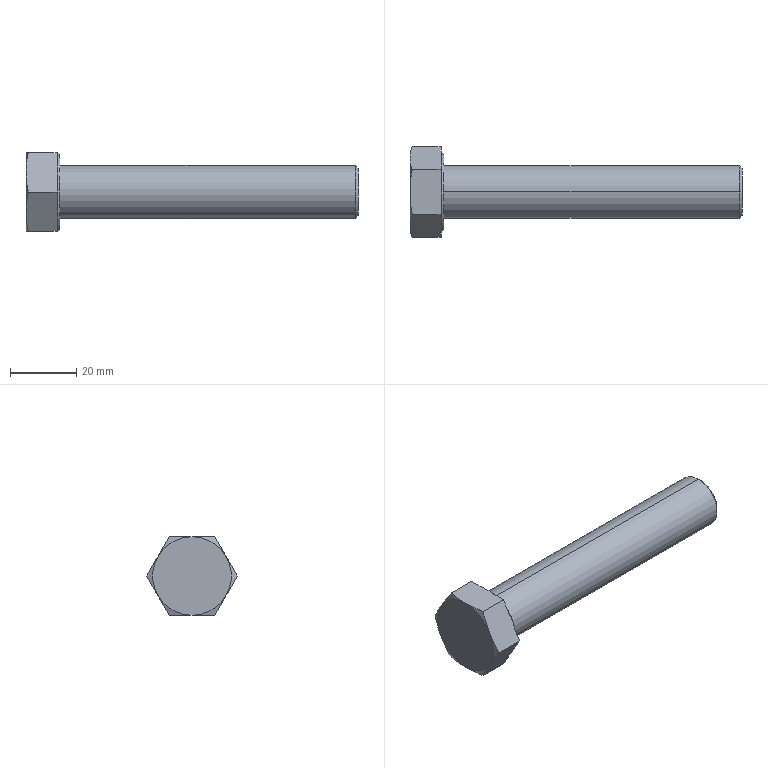Part | SolidWorks | features RevCut 3, Boss 1, Chamfer 1, Extrusion 1, Fillet 1, LPattern 1 | 1 solid | 27 faces | box 100.18 x 27.332 x 23.67 mm | volume 22963 mm3 | plane 15 | cone 10 | cylinder 2 | commonest cylinder face diameters 16 x2
STEP:
#1=CARTESIAN_POINT('',(100.18,0.,-7.2));
#2=VERTEX_POINT('',#1);
#3=CARTESIAN_POINT('',(100.18,0.,7.2));
#4=VERTEX_POINT('',#3);
#5=CARTESIAN_POINT('',(100.18,0.,0.));
#6=DIRECTION('',(1.,0.,0.));
#7=DIRECTION('',(0.,0.,-1.));
#8=AXIS2_PLACEMENT_3D('',#5,#6,#7);
#9=CIRCLE('',#8,7.2);
#10=EDGE_CURVE('',#2,#4,#9,.T.);
#11=ORIENTED_EDGE('',*,*,#10,.F.);
#12=CARTESIAN_POINT('',(99.38,0.,-8.));
#13=VERTEX_POINT('',#12);
#14=CARTESIAN_POINT('',(100.18,0.,-7.2));
#15=DIRECTION('',(-0.7071,0.,-0.7071));
#16=VECTOR('',#15,1000.);
#17=LINE('',#14,#16);
#18=EDGE_CURVE('',#2,#13,#17,.T.);
#19=ORIENTED_EDGE('',*,*,#18,.T.);
#20=CARTESIAN_POINT('',(99.38,0.,8.));
#21=VERTEX_POINT('',#20);
#22=CARTESIAN_POINT('',(99.38,0.,0.));
#23=DIRECTION('',(-1.,0.,0.));
#24=DIRECTION('',(0.,0.,-1.));
#25=AXIS2_PLACEMENT_3D('',#22,#23,#24);
#26=CIRCLE('',#25,8.);
#27=EDGE_CURVE('',#21,#13,#26,.T.);
#28=ORIENTED_EDGE('',*,*,#27,.F.);
#29=CARTESIAN_POINT('',(100.18,0.,7.2));
#30=DIRECTION('',(-0.7071,0.,0.7071));
#31=VECTOR('',#30,1000.);
#32=LINE('',#29,#31);
#33=EDGE_CURVE('',#4,#21,#32,.T.);
#34=ORIENTED_EDGE('',*,*,#33,.F.);
#35=EDGE_LOOP('',(#11,#19,#28,#34));
#36=FACE_OUTER_BOUND('',#35,.T.);
#37=CARTESIAN_POINT('',(100.18,0.,0.));
#38=DIRECTION('',(-1.,0.,0.));
#39=DIRECTION('',(0.,0.,1.));
#40=AXIS2_PLACEMENT_3D('',#37,#38,#39);
#41=CONICAL_SURFACE('',#40,7.2,0.7854);
#42=ADVANCED_FACE('',(#36),#41,.T.);
#43=ORIENTED_EDGE('',*,*,#27,.T.);
#44=CARTESIAN_POINT('',(10.18,0.,-8.));
#45=VERTEX_POINT('',#44);
#46=CARTESIAN_POINT('',(100.18,0.,-8.));
#47=DIRECTION('',(-1.,0.,0.));
#48=VECTOR('',#47,1000.);
#49=LINE('',#46,#48);
#50=EDGE_CURVE('',#13,#45,#49,.T.);
#51=ORIENTED_EDGE('',*,*,#50,.T.);
#52=CARTESIAN_POINT('',(10.18,0.,8.));
#53=VERTEX_POINT('',#52);
#54=CARTESIAN_POINT('',(10.18,0.,0.));
#55=DIRECTION('',(1.,0.,0.));
#56=DIRECTION('',(0.,0.,-1.));
#57=AXIS2_PLACEMENT_3D('',#54,#55,#56);
#58=CIRCLE('',#57,8.);
#59=EDGE_CURVE('',#45,#53,#58,.T.);
#60=ORIENTED_EDGE('',*,*,#59,.T.);
#61=CARTESIAN_POINT('',(100.18,0.,8.));
#62=DIRECTION('',(-1.,0.,0.));
#63=VECTOR('',#62,1000.);
#64=LINE('',#61,#63);
#65=EDGE_CURVE('',#21,#53,#64,.T.);
#66=ORIENTED_EDGE('',*,*,#65,.F.);
#67=EDGE_LOOP('',(#43,#51,#60,#66));
#68=FACE_OUTER_BOUND('',#67,.T.);
#69=CARTESIAN_POINT('',(100.18,0.,0.));
#70=DIRECTION('',(-1.,0.,0.));
#71=DIRECTION('',(0.,0.,1.));
#72=AXIS2_PLACEMENT_3D('',#69,#70,#71);
#73=CYLINDRICAL_SURFACE('',#72,8.);
#74=ADVANCED_FACE('',(#68),#73,.T.);
#75=CARTESIAN_POINT('',(10.18,0.,11.245));
#76=VERTEX_POINT('',#75);
#77=CARTESIAN_POINT('',(10.18,0.,-11.245));
#78=VERTEX_POINT('',#77);
#79=CARTESIAN_POINT('',(10.18,0.,0.));
#80=DIRECTION('',(-1.,0.,0.));
#81=DIRECTION('',(0.,0.,1.));
#82=AXIS2_PLACEMENT_3D('',#79,#80,#81);
#83=CIRCLE('',#82,11.245);
#84=EDGE_CURVE('',#76,#78,#83,.T.);
#85=ORIENTED_EDGE('',*,*,#84,.T.);
#86=CARTESIAN_POINT('',(9.59,0.,-11.835));
#87=VERTEX_POINT('',#86);
#88=CARTESIAN_POINT('',(9.38,0.,-12.045));
#89=DIRECTION('',(-0.7071,0.,-0.7071));
#90=VECTOR('',#89,1000.);
#91=LINE('',#88,#90);
#92=EDGE_CURVE('',#78,#87,#91,.T.);
#93=ORIENTED_EDGE('',*,*,#92,.T.);
#94=CARTESIAN_POINT('',(9.38,2.239,-11.835));
#95=VERTEX_POINT('',#94);
#96=CARTESIAN_POINT('',(9.59,0.,-11.835));
#97=CARTESIAN_POINT('',(9.59,0.3738,-11.835));
#98=CARTESIAN_POINT('',(9.572,0.7475,-11.835));
#99=CARTESIAN_POINT('',(9.502,1.495,-11.835));
#100=CARTESIAN_POINT('',(9.449,1.87,-11.835));
#101=CARTESIAN_POINT('',(9.38,2.239,-11.835));
#102=B_SPLINE_CURVE_WITH_KNOTS('',3,(#96,#97,#98,#99,#100,#101),.UNSPECIFIED.,.F.,.F.,(4,2,4),(0.00667,0.007787,0.008904),.UNSPECIFIED.);
#103=EDGE_CURVE('',#87,#95,#102,.T.);
#104=ORIENTED_EDGE('',*,*,#103,.T.);
#105=CARTESIAN_POINT('',(9.38,9.13,-7.857));
#106=VERTEX_POINT('',#105);
#107=CARTESIAN_POINT('',(9.38,0.,0.));
#108=DIRECTION('',(-1.,0.,0.));
#109=DIRECTION('',(0.,0.,1.));
#110=AXIS2_PLACEMENT_3D('',#107,#108,#109);
#111=CIRCLE('',#110,12.045);
#112=EDGE_CURVE('',#106,#95,#111,.T.);
#113=ORIENTED_EDGE('',*,*,#112,.F.);
#114=CARTESIAN_POINT('',(9.38,11.369,-3.978));
#115=VERTEX_POINT('',#114);
#116=CARTESIAN_POINT('',(9.38,9.13,-7.857));
#117=CARTESIAN_POINT('',(9.518,9.501,-7.214));
#118=CARTESIAN_POINT('',(9.59,9.873,-6.569));
#119=CARTESIAN_POINT('',(9.59,10.621,-5.274));
#120=CARTESIAN_POINT('',(9.518,10.998,-4.621));
#121=CARTESIAN_POINT('',(9.38,11.369,-3.978));
#122=B_SPLINE_CURVE_WITH_KNOTS('',3,(#116,#117,#118,#119,#120,#121),.UNSPECIFIED.,.F.,.F.,(4,2,4),(0.000001082,0.002242,0.004483),.UNSPECIFIED.);
#123=EDGE_CURVE('',#106,#115,#122,.T.);
#124=ORIENTED_EDGE('',*,*,#123,.T.);
#125=CARTESIAN_POINT('',(9.38,11.369,3.978));
#126=VERTEX_POINT('',#125);
#127=CARTESIAN_POINT('',(9.38,0.,0.));
#128=DIRECTION('',(-1.,0.,0.));
#129=DIRECTION('',(0.,0.,1.));
#130=AXIS2_PLACEMENT_3D('',#127,#128,#129);
#131=CIRCLE('',#130,12.045);
#132=EDGE_CURVE('',#126,#115,#131,.T.);
#133=ORIENTED_EDGE('',*,*,#132,.F.);
#134=CARTESIAN_POINT('',(9.38,9.13,7.857));
#135=VERTEX_POINT('',#134);
#136=CARTESIAN_POINT('',(9.38,11.369,3.978));
#137=CARTESIAN_POINT('',(9.518,10.998,4.621));
#138=CARTESIAN_POINT('',(9.59,10.626,5.266));
#139=CARTESIAN_POINT('',(9.59,9.878,6.561));
#140=CARTESIAN_POINT('',(9.518,9.501,7.214));
#141=CARTESIAN_POINT('',(9.38,9.13,7.857));
#142=B_SPLINE_CURVE_WITH_KNOTS('',3,(#136,#137,#138,#139,#140,#141),.UNSPECIFIED.,.F.,.F.,(4,2,4),(0.000001082,0.002242,0.004483),.UNSPECIFIED.);
#143=EDGE_CURVE('',#126,#135,#142,.T.);
#144=ORIENTED_EDGE('',*,*,#143,.T.);
#145=CARTESIAN_POINT('',(9.38,2.239,11.835));
#146=VERTEX_POINT('',#145);
#147=CARTESIAN_POINT('',(9.38,0.,0.));
#148=DIRECTION('',(-1.,0.,0.));
#149=DIRECTION('',(0.,0.,1.));
#150=AXIS2_PLACEMENT_3D('',#147,#148,#149);
#151=CIRCLE('',#150,12.045);
#152=EDGE_CURVE('',#146,#135,#151,.T.);
#153=ORIENTED_EDGE('',*,*,#152,.F.);
#154=CARTESIAN_POINT('',(9.59,0.,11.835));
#155=VERTEX_POINT('',#154);
#156=CARTESIAN_POINT('',(9.38,2.239,11.835));
#157=CARTESIAN_POINT('',(9.449,1.87,11.835));
#158=CARTESIAN_POINT('',(9.502,1.495,11.835));
#159=CARTESIAN_POINT('',(9.572,0.7475,11.835));
#160=CARTESIAN_POINT('',(9.59,0.3738,11.835));
#161=CARTESIAN_POINT('',(9.59,0.,11.835));
#162=B_SPLINE_CURVE_WITH_KNOTS('',3,(#156,#157,#158,#159,#160,#161),.UNSPECIFIED.,.F.,.F.,(4,2,4),(0.004938,0.006055,0.007171),.UNSPECIFIED.);
#163=EDGE_CURVE('',#146,#155,#162,.T.);
#164=ORIENTED_EDGE('',*,*,#163,.T.);
#165=CARTESIAN_POINT('',(9.38,0.,12.045));
#166=DIRECTION('',(-0.7071,0.,0.7071));
#167=VECTOR('',#166,1000.);
#168=LINE('',#165,#167);
#169=EDGE_CURVE('',#76,#155,#168,.T.);
#170=ORIENTED_EDGE('',*,*,#169,.F.);
#171=EDGE_LOOP('',(#85,#93,#104,#113,#124,#133,#144,#153,#164,#170));
#172=FACE_OUTER_BOUND('',#171,.T.);
#173=CARTESIAN_POINT('',(9.38,0.,0.));
#174=DIRECTION('',(-1.,0.,0.));
#175=DIRECTION('',(0.,0.,1.));
#176=AXIS2_PLACEMENT_3D('',#173,#174,#175);
#177=CONICAL_SURFACE('',#176,12.045,0.7854);
#178=ADVANCED_FACE('',(#172),#177,.T.);
#179=ORIENTED_EDGE('',*,*,#84,.F.);
#180=CARTESIAN_POINT('',(10.18,0.,0.));
#181=DIRECTION('',(-1.,0.,0.));
#182=DIRECTION('',(0.,0.,1.));
#183=AXIS2_PLACEMENT_3D('',#180,#181,#182);
#184=CIRCLE('',#183,11.245);
#185=EDGE_CURVE('',#78,#76,#184,.T.);
#186=ORIENTED_EDGE('',*,*,#185,.F.);
#187=EDGE_LOOP('',(#179,#186));
#188=FACE_OUTER_BOUND('',#187,.T.);
#189=CARTESIAN_POINT('',(10.18,0.,0.));
#190=DIRECTION('',(1.,0.,0.));
#191=DIRECTION('',(0.,0.,-1.));
#192=AXIS2_PLACEMENT_3D('',#189,#190,#191);
#193=CIRCLE('',#192,8.);
#194=EDGE_CURVE('',#53,#45,#193,.T.);
#195=ORIENTED_EDGE('',*,*,#194,.F.);
#196=ORIENTED_EDGE('',*,*,#59,.F.);
#197=EDGE_LOOP('',(#195,#196));
#198=FACE_BOUND('',#197,.T.);
#199=CARTESIAN_POINT('',(10.18,-6.833,-11.835));
#200=DIRECTION('',(1.,0.,0.));
#201=DIRECTION('',(0.,0.,-1.));
#202=AXIS2_PLACEMENT_3D('',#199,#200,#201);
#203=PLANE('',#202);
#204=ADVANCED_FACE('',(#188,#198),#203,.T.);
#205=CARTESIAN_POINT('',(0.6664,-6.833,-11.835));
#206=VERTEX_POINT('',#205);
#207=CARTESIAN_POINT('',(0.,-10.249,-5.917));
#208=VERTEX_POINT('',#207);
#209=CARTESIAN_POINT('',(0.6664,-6.833,-11.835));
#210=CARTESIAN_POINT('',(0.4591,-7.402,-10.849));
#211=CARTESIAN_POINT('',(0.2909,-7.972,-9.862));
#212=CARTESIAN_POINT('',(0.06093,-9.111,-7.89));
#213=CARTESIAN_POINT('',(0.,-9.68,-6.904));
#214=CARTESIAN_POINT('',(0.,-10.249,-5.917));
#215=B_SPLINE_CURVE_WITH_KNOTS('',3,(#209,#210,#211,#212,#213,#214),.UNSPECIFIED.,.F.,.F.,(4,2,4),(0.000000231,0.003417,0.006833),.UNSPECIFIED.);
#216=EDGE_CURVE('',#206,#208,#215,.T.);
#217=ORIENTED_EDGE('',*,*,#216,.F.);
#218=CARTESIAN_POINT('',(9.38,-6.833,-11.835));
#219=VERTEX_POINT('',#218);
#220=CARTESIAN_POINT('',(10.18,-6.833,-11.835));
#221=DIRECTION('',(-1.,0.,0.));
#222=VECTOR('',#221,1000.);
#223=LINE('',#220,#222);
#224=EDGE_CURVE('',#219,#206,#223,.T.);
#225=ORIENTED_EDGE('',*,*,#224,.F.);
#226=CARTESIAN_POINT('',(9.38,-9.13,-7.857));
#227=VERTEX_POINT('',#226);
#228=CARTESIAN_POINT('',(9.38,-13.666,0.));
#229=DIRECTION('',(0.,0.5,-0.866));
#230=VECTOR('',#229,1000.);
#231=LINE('',#228,#230);
#232=EDGE_CURVE('',#227,#219,#231,.T.);
#233=ORIENTED_EDGE('',*,*,#232,.F.);
#234=CARTESIAN_POINT('',(9.38,-11.369,-3.978));
#235=VERTEX_POINT('',#234);
#236=CARTESIAN_POINT('',(9.38,-11.369,-3.978));
#237=CARTESIAN_POINT('',(9.518,-10.998,-4.621));
#238=CARTESIAN_POINT('',(9.59,-10.626,-5.266));
#239=CARTESIAN_POINT('',(9.59,-9.878,-6.561));
#240=CARTESIAN_POINT('',(9.518,-9.501,-7.214));
#241=CARTESIAN_POINT('',(9.38,-9.13,-7.857));
#242=B_SPLINE_CURVE_WITH_KNOTS('',3,(#236,#237,#238,#239,#240,#241),.UNSPECIFIED.,.F.,.F.,(4,2,4),(0.000001082,0.002242,0.004483),.UNSPECIFIED.);
#243=EDGE_CURVE('',#235,#227,#242,.T.);
#244=ORIENTED_EDGE('',*,*,#243,.F.);
#245=CARTESIAN_POINT('',(9.38,-13.666,0.));
#246=VERTEX_POINT('',#245);
#247=CARTESIAN_POINT('',(9.38,-13.666,0.));
#248=DIRECTION('',(0.,0.5,-0.866));
#249=VECTOR('',#248,1000.);
#250=LINE('',#247,#249);
#251=EDGE_CURVE('',#246,#235,#250,.T.);
#252=ORIENTED_EDGE('',*,*,#251,.F.);
#253=CARTESIAN_POINT('',(0.6664,-13.666,0.));
#254=VERTEX_POINT('',#253);
#255=CARTESIAN_POINT('',(10.18,-13.666,0.));
#256=DIRECTION('',(-1.,0.,0.));
#257=VECTOR('',#256,1000.);
#258=LINE('',#255,#257);
#259=EDGE_CURVE('',#246,#254,#258,.T.);
#260=ORIENTED_EDGE('',*,*,#259,.T.);
#261=CARTESIAN_POINT('',(0.,-10.249,-5.917));
#262=CARTESIAN_POINT('',(0.,-10.819,-4.931));
#263=CARTESIAN_POINT('',(0.06093,-11.388,-3.945));
#264=CARTESIAN_POINT('',(0.2909,-12.527,-1.972));
#265=CARTESIAN_POINT('',(0.4591,-13.096,-0.9862));
#266=CARTESIAN_POINT('',(0.6664,-13.666,0.));
#267=B_SPLINE_CURVE_WITH_KNOTS('',3,(#261,#262,#263,#264,#265,#266),.UNSPECIFIED.,.F.,.F.,(4,2,4),(0.006833,0.01025,0.01367),.UNSPECIFIED.);
#268=EDGE_CURVE('',#208,#254,#267,.T.);
#269=ORIENTED_EDGE('',*,*,#268,.F.);
#270=EDGE_LOOP('',(#217,#225,#233,#244,#252,#260,#269));
#271=FACE_OUTER_BOUND('',#270,.T.);
#272=CARTESIAN_POINT('',(10.18,-13.666,0.));
#273=DIRECTION('',(0.,0.866,0.5));
#274=DIRECTION('',(0.,-0.5,0.866));
#275=AXIS2_PLACEMENT_3D('',#272,#273,#274);
#276=PLANE('',#275);
#277=ADVANCED_FACE('',(#271),#276,.F.);
#278=CARTESIAN_POINT('',(0.6664,6.833,-11.835));
#279=VERTEX_POINT('',#278);
#280=CARTESIAN_POINT('',(0.,0.,-11.835));
#281=VERTEX_POINT('',#280);
#282=CARTESIAN_POINT('',(0.6664,6.833,-11.835));
#283=CARTESIAN_POINT('',(0.4597,5.697,-11.835));
#284=CARTESIAN_POINT('',(0.2913,4.559,-11.835));
#285=CARTESIAN_POINT('',(0.06117,2.281,-11.835));
#286=CARTESIAN_POINT('',(0.,1.141,-11.835));
#287=CARTESIAN_POINT('',(0.,0.,-11.835));
#288=B_SPLINE_CURVE_WITH_KNOTS('',3,(#282,#283,#284,#285,#286,#287),.UNSPECIFIED.,.F.,.F.,(4,2,4),(0.02464,0.02808,0.03153),.UNSPECIFIED.);
#289=EDGE_CURVE('',#279,#281,#288,.T.);
#290=ORIENTED_EDGE('',*,*,#289,.F.);
#291=CARTESIAN_POINT('',(9.38,6.833,-11.835));
#292=VERTEX_POINT('',#291);
#293=CARTESIAN_POINT('',(10.18,6.833,-11.835));
#294=DIRECTION('',(-1.,0.,0.));
#295=VECTOR('',#294,1000.);
#296=LINE('',#293,#295);
#297=EDGE_CURVE('',#292,#279,#296,.T.);
#298=ORIENTED_EDGE('',*,*,#297,.F.);
#299=CARTESIAN_POINT('',(9.38,-6.833,-11.835));
#300=DIRECTION('',(0.,1.,0.));
#301=VECTOR('',#300,1000.);
#302=LINE('',#299,#301);
#303=EDGE_CURVE('',#95,#292,#302,.T.);
#304=ORIENTED_EDGE('',*,*,#303,.F.);
#305=ORIENTED_EDGE('',*,*,#103,.F.);
#306=CARTESIAN_POINT('',(9.38,-2.239,-11.835));
#307=VERTEX_POINT('',#306);
#308=CARTESIAN_POINT('',(9.38,-2.239,-11.835));
#309=CARTESIAN_POINT('',(9.449,-1.871,-11.835));
#310=CARTESIAN_POINT('',(9.502,-1.495,-11.835));
#311=CARTESIAN_POINT('',(9.572,-0.7474,-11.835));
#312=CARTESIAN_POINT('',(9.59,-0.3736,-11.835));
#313=CARTESIAN_POINT('',(9.59,0.,-11.835));
#314=B_SPLINE_CURVE_WITH_KNOTS('',3,(#308,#309,#310,#311,#312,#313),.UNSPECIFIED.,.F.,.F.,(4,2,4),(0.004436,0.005553,0.00667),.UNSPECIFIED.);
#315=EDGE_CURVE('',#307,#87,#314,.T.);
#316=ORIENTED_EDGE('',*,*,#315,.F.);
#317=CARTESIAN_POINT('',(9.38,-6.833,-11.835));
#318=DIRECTION('',(0.,1.,0.));
#319=VECTOR('',#318,1000.);
#320=LINE('',#317,#319);
#321=EDGE_CURVE('',#219,#307,#320,.T.);
#322=ORIENTED_EDGE('',*,*,#321,.F.);
#323=ORIENTED_EDGE('',*,*,#224,.T.);
#324=CARTESIAN_POINT('',(0.,0.,-11.835));
#325=CARTESIAN_POINT('',(0.,-1.138,-11.835));
#326=CARTESIAN_POINT('',(0.06084,-2.277,-11.835));
#327=CARTESIAN_POINT('',(0.2911,-4.558,-11.835));
#328=CARTESIAN_POINT('',(0.4605,-5.702,-11.835));
#329=CARTESIAN_POINT('',(0.6664,-6.833,-11.835));
#330=B_SPLINE_CURVE_WITH_KNOTS('',3,(#324,#325,#326,#327,#328,#329),.UNSPECIFIED.,.F.,.F.,(4,2,4),(0.03153,0.03496,0.0384),.UNSPECIFIED.);
#331=EDGE_CURVE('',#281,#206,#330,.T.);
#332=ORIENTED_EDGE('',*,*,#331,.F.);
#333=EDGE_LOOP('',(#290,#298,#304,#305,#316,#322,#323,#332));
#334=FACE_OUTER_BOUND('',#333,.T.);
#335=CARTESIAN_POINT('',(10.18,-6.833,-11.835));
#336=DIRECTION('',(0.,0.,1.));
#337=DIRECTION('',(1.,0.,0.));
#338=AXIS2_PLACEMENT_3D('',#335,#336,#337);
#339=PLANE('',#338);
#340=ADVANCED_FACE('',(#334),#339,.F.);
#341=CARTESIAN_POINT('',(0.6664,13.666,0.));
#342=VERTEX_POINT('',#341);
#343=CARTESIAN_POINT('',(0.,10.249,-5.917));
#344=VERTEX_POINT('',#343);
#345=CARTESIAN_POINT('',(0.6664,13.666,0.));
#346=CARTESIAN_POINT('',(0.4591,13.096,-0.9862));
#347=CARTESIAN_POINT('',(0.2909,12.527,-1.972));
#348=CARTESIAN_POINT('',(0.06093,11.388,-3.945));
#349=CARTESIAN_POINT('',(0.,10.819,-4.931));
#350=CARTESIAN_POINT('',(0.,10.249,-5.917));
#351=B_SPLINE_CURVE_WITH_KNOTS('',3,(#345,#346,#347,#348,#349,#350),.UNSPECIFIED.,.F.,.F.,(4,2,4),(0.000000231,0.003417,0.006833),.UNSPECIFIED.);
#352=EDGE_CURVE('',#342,#344,#351,.T.);
#353=ORIENTED_EDGE('',*,*,#352,.F.);
#354=CARTESIAN_POINT('',(9.38,13.666,0.));
#355=VERTEX_POINT('',#354);
#356=CARTESIAN_POINT('',(10.18,13.666,0.));
#357=DIRECTION('',(-1.,0.,0.));
#358=VECTOR('',#357,1000.);
#359=LINE('',#356,#358);
#360=EDGE_CURVE('',#355,#342,#359,.T.);
#361=ORIENTED_EDGE('',*,*,#360,.F.);
#362=CARTESIAN_POINT('',(9.38,6.833,-11.835));
#363=DIRECTION('',(0.,0.5,0.866));
#364=VECTOR('',#363,1000.);
#365=LINE('',#362,#364);
#366=EDGE_CURVE('',#115,#355,#365,.T.);
#367=ORIENTED_EDGE('',*,*,#366,.F.);
#368=ORIENTED_EDGE('',*,*,#123,.F.);
#369=CARTESIAN_POINT('',(9.38,6.833,-11.835));
#370=DIRECTION('',(0.,0.5,0.866));
#371=VECTOR('',#370,1000.);
#372=LINE('',#369,#371);
#373=EDGE_CURVE('',#292,#106,#372,.T.);
#374=ORIENTED_EDGE('',*,*,#373,.F.);
#375=ORIENTED_EDGE('',*,*,#297,.T.);
#376=CARTESIAN_POINT('',(0.,10.249,-5.917));
#377=CARTESIAN_POINT('',(0.,9.68,-6.904));
#378=CARTESIAN_POINT('',(0.06093,9.111,-7.89));
#379=CARTESIAN_POINT('',(0.2909,7.972,-9.862));
#380=CARTESIAN_POINT('',(0.4591,7.402,-10.849));
#381=CARTESIAN_POINT('',(0.6664,6.833,-11.835));
#382=B_SPLINE_CURVE_WITH_KNOTS('',3,(#376,#377,#378,#379,#380,#381),.UNSPECIFIED.,.F.,.F.,(4,2,4),(0.006833,0.01025,0.01367),.UNSPECIFIED.);
#383=EDGE_CURVE('',#344,#279,#382,.T.);
#384=ORIENTED_EDGE('',*,*,#383,.F.);
#385=EDGE_LOOP('',(#353,#361,#367,#368,#374,#375,#384));
#386=FACE_OUTER_BOUND('',#385,.T.);
#387=CARTESIAN_POINT('',(10.18,6.833,-11.835));
#388=DIRECTION('',(0.,-0.866,0.5));
#389=DIRECTION('',(0.,-0.5,-0.866));
#390=AXIS2_PLACEMENT_3D('',#387,#388,#389);
#391=PLANE('',#390);
#392=ADVANCED_FACE('',(#386),#391,.F.);
#393=CARTESIAN_POINT('',(0.6664,6.833,11.835));
#394=VERTEX_POINT('',#393);
#395=CARTESIAN_POINT('',(0.,10.249,5.917));
#396=VERTEX_POINT('',#395);
#397=CARTESIAN_POINT('',(0.6664,6.833,11.835));
#398=CARTESIAN_POINT('',(0.4591,7.402,10.849));
#399=CARTESIAN_POINT('',(0.2909,7.972,9.863));
#400=CARTESIAN_POINT('',(0.06093,9.111,7.89));
#401=CARTESIAN_POINT('',(0.,9.68,6.904));
#402=CARTESIAN_POINT('',(0.,10.249,5.917));
#403=B_SPLINE_CURVE_WITH_KNOTS('',3,(#397,#398,#399,#400,#401,#402),.UNSPECIFIED.,.F.,.F.,(4,2,4),(0.000000231,0.003417,0.006833),.UNSPECIFIED.);
#404=EDGE_CURVE('',#394,#396,#403,.T.);
#405=ORIENTED_EDGE('',*,*,#404,.F.);
#406=CARTESIAN_POINT('',(9.38,6.833,11.835));
#407=VERTEX_POINT('',#406);
#408=CARTESIAN_POINT('',(10.18,6.833,11.835));
#409=DIRECTION('',(-1.,0.,0.));
#410=VECTOR('',#409,1000.);
#411=LINE('',#408,#410);
#412=EDGE_CURVE('',#407,#394,#411,.T.);
#413=ORIENTED_EDGE('',*,*,#412,.F.);
#414=CARTESIAN_POINT('',(9.38,13.666,0.));
#415=DIRECTION('',(0.,-0.5,0.866));
#416=VECTOR('',#415,1000.);
#417=LINE('',#414,#416);
#418=EDGE_CURVE('',#135,#407,#417,.T.);
#419=ORIENTED_EDGE('',*,*,#418,.F.);
#420=ORIENTED_EDGE('',*,*,#143,.F.);
#421=CARTESIAN_POINT('',(9.38,13.666,0.));
#422=DIRECTION('',(0.,-0.5,0.866));
#423=VECTOR('',#422,1000.);
#424=LINE('',#421,#423);
#425=EDGE_CURVE('',#355,#126,#424,.T.);
#426=ORIENTED_EDGE('',*,*,#425,.F.);
#427=ORIENTED_EDGE('',*,*,#360,.T.);
#428=CARTESIAN_POINT('',(0.,10.249,5.917));
#429=CARTESIAN_POINT('',(0.,10.819,4.931));
#430=CARTESIAN_POINT('',(0.06093,11.388,3.945));
#431=CARTESIAN_POINT('',(0.2909,12.527,1.972));
#432=CARTESIAN_POINT('',(0.4591,13.096,0.9862));
#433=CARTESIAN_POINT('',(0.6664,13.666,0.));
#434=B_SPLINE_CURVE_WITH_KNOTS('',3,(#428,#429,#430,#431,#432,#433),.UNSPECIFIED.,.F.,.F.,(4,2,4),(0.006833,0.01025,0.01367),.UNSPECIFIED.);
#435=EDGE_CURVE('',#396,#342,#434,.T.);
#436=ORIENTED_EDGE('',*,*,#435,.F.);
#437=EDGE_LOOP('',(#405,#413,#419,#420,#426,#427,#436));
#438=FACE_OUTER_BOUND('',#437,.T.);
#439=CARTESIAN_POINT('',(10.18,13.666,0.));
#440=DIRECTION('',(0.,-0.866,-0.5));
#441=DIRECTION('',(0.,0.5,-0.866));
#442=AXIS2_PLACEMENT_3D('',#439,#440,#441);
#443=PLANE('',#442);
#444=ADVANCED_FACE('',(#438),#443,.F.);
#445=CARTESIAN_POINT('',(0.6664,-6.833,11.835));
#446=VERTEX_POINT('',#445);
#447=CARTESIAN_POINT('',(0.,0.,11.835));
#448=VERTEX_POINT('',#447);
#449=CARTESIAN_POINT('',(0.6664,-6.833,11.835));
#450=CARTESIAN_POINT('',(0.4605,-5.702,11.835));
#451=CARTESIAN_POINT('',(0.2911,-4.558,11.835));
#452=CARTESIAN_POINT('',(0.06084,-2.277,11.835));
#453=CARTESIAN_POINT('',(0.,-1.138,11.835));
#454=CARTESIAN_POINT('',(0.,0.,11.835));
#455=B_SPLINE_CURVE_WITH_KNOTS('',3,(#449,#450,#451,#452,#453,#454),.UNSPECIFIED.,.F.,.F.,(4,2,4),(0.01162,0.01507,0.01851),.UNSPECIFIED.);
#456=EDGE_CURVE('',#446,#448,#455,.T.);
#457=ORIENTED_EDGE('',*,*,#456,.F.);
#458=CARTESIAN_POINT('',(9.38,-6.833,11.835));
#459=VERTEX_POINT('',#458);
#460=CARTESIAN_POINT('',(10.18,-6.833,11.835));
#461=DIRECTION('',(-1.,0.,0.));
#462=VECTOR('',#461,1000.);
#463=LINE('',#460,#462);
#464=EDGE_CURVE('',#459,#446,#463,.T.);
#465=ORIENTED_EDGE('',*,*,#464,.F.);
#466=CARTESIAN_POINT('',(9.38,-2.239,11.835));
#467=VERTEX_POINT('',#466);
#468=CARTESIAN_POINT('',(9.38,6.833,11.835));
#469=DIRECTION('',(0.,-1.,0.));
#470=VECTOR('',#469,1000.);
#471=LINE('',#468,#470);
#472=EDGE_CURVE('',#467,#459,#471,.T.);
#473=ORIENTED_EDGE('',*,*,#472,.F.);
#474=CARTESIAN_POINT('',(9.59,0.,11.835));
#475=CARTESIAN_POINT('',(9.59,-0.3736,11.835));
#476=CARTESIAN_POINT('',(9.572,-0.7474,11.835));
#477=CARTESIAN_POINT('',(9.502,-1.495,11.835));
#478=CARTESIAN_POINT('',(9.449,-1.871,11.835));
#479=CARTESIAN_POINT('',(9.38,-2.239,11.835));
#480=B_SPLINE_CURVE_WITH_KNOTS('',3,(#474,#475,#476,#477,#478,#479),.UNSPECIFIED.,.F.,.F.,(4,2,4),(0.007171,0.008287,0.009403),.UNSPECIFIED.);
#481=EDGE_CURVE('',#155,#467,#480,.T.);
#482=ORIENTED_EDGE('',*,*,#481,.F.);
#483=ORIENTED_EDGE('',*,*,#163,.F.);
#484=CARTESIAN_POINT('',(9.38,6.833,11.835));
#485=DIRECTION('',(0.,-1.,0.));
#486=VECTOR('',#485,1000.);
#487=LINE('',#484,#486);
#488=EDGE_CURVE('',#407,#146,#487,.T.);
#489=ORIENTED_EDGE('',*,*,#488,.F.);
#490=ORIENTED_EDGE('',*,*,#412,.T.);
#491=CARTESIAN_POINT('',(0.,0.,11.835));
#492=CARTESIAN_POINT('',(0.,1.141,11.835));
#493=CARTESIAN_POINT('',(0.06117,2.281,11.835));
#494=CARTESIAN_POINT('',(0.2913,4.559,11.835));
#495=CARTESIAN_POINT('',(0.4597,5.697,11.835));
#496=CARTESIAN_POINT('',(0.6664,6.833,11.835));
#497=B_SPLINE_CURVE_WITH_KNOTS('',3,(#491,#492,#493,#494,#495,#496),.UNSPECIFIED.,.F.,.F.,(4,2,4),(0.01851,0.02196,0.02542),.UNSPECIFIED.);
#498=EDGE_CURVE('',#448,#394,#497,.T.);
#499=ORIENTED_EDGE('',*,*,#498,.F.);
#500=EDGE_LOOP('',(#457,#465,#473,#482,#483,#489,#490,#499));
#501=FACE_OUTER_BOUND('',#500,.T.);
#502=CARTESIAN_POINT('',(10.18,6.833,11.835));
#503=DIRECTION('',(0.,0.,-1.));
#504=DIRECTION('',(-1.,0.,0.));
#505=AXIS2_PLACEMENT_3D('',#502,#503,#504);
#506=PLANE('',#505);
#507=ADVANCED_FACE('',(#501),#506,.F.);
#508=CARTESIAN_POINT('',(0.,-10.249,5.918));
#509=VERTEX_POINT('',#508);
#510=CARTESIAN_POINT('',(0.6664,-13.666,0.));
#511=CARTESIAN_POINT('',(0.4591,-13.096,0.9863));
#512=CARTESIAN_POINT('',(0.2909,-12.527,1.973));
#513=CARTESIAN_POINT('',(0.06093,-11.388,3.945));
#514=CARTESIAN_POINT('',(0.,-10.819,4.931));
#515=CARTESIAN_POINT('',(0.,-10.249,5.918));
#516=B_SPLINE_CURVE_WITH_KNOTS('',3,(#510,#511,#512,#513,#514,#515),.UNSPECIFIED.,.F.,.F.,(4,2,4),(0.000000231,0.003417,0.006833),.UNSPECIFIED.);
#517=EDGE_CURVE('',#254,#509,#516,.T.);
#518=ORIENTED_EDGE('',*,*,#517,.F.);
#519=ORIENTED_EDGE('',*,*,#259,.F.);
#520=CARTESIAN_POINT('',(9.38,-11.369,3.978));
#521=VERTEX_POINT('',#520);
#522=CARTESIAN_POINT('',(9.38,-6.833,11.835));
#523=DIRECTION('',(0.,-0.5,-0.866));
#524=VECTOR('',#523,1000.);
#525=LINE('',#522,#524);
#526=EDGE_CURVE('',#521,#246,#525,.T.);
#527=ORIENTED_EDGE('',*,*,#526,.F.);
#528=CARTESIAN_POINT('',(9.38,-9.13,7.857));
#529=VERTEX_POINT('',#528);
#530=CARTESIAN_POINT('',(9.38,-9.13,7.857));
#531=CARTESIAN_POINT('',(9.518,-9.501,7.214));
#532=CARTESIAN_POINT('',(9.59,-9.873,6.569));
#533=CARTESIAN_POINT('',(9.59,-10.621,5.274));
#534=CARTESIAN_POINT('',(9.518,-10.998,4.621));
#535=CARTESIAN_POINT('',(9.38,-11.369,3.978));
#536=B_SPLINE_CURVE_WITH_KNOTS('',3,(#530,#531,#532,#533,#534,#535),.UNSPECIFIED.,.F.,.F.,(4,2,4),(0.000001082,0.002242,0.004483),.UNSPECIFIED.);
#537=EDGE_CURVE('',#529,#521,#536,.T.);
#538=ORIENTED_EDGE('',*,*,#537,.F.);
#539=CARTESIAN_POINT('',(9.38,-6.833,11.835));
#540=DIRECTION('',(0.,-0.5,-0.866));
#541=VECTOR('',#540,1000.);
#542=LINE('',#539,#541);
#543=EDGE_CURVE('',#459,#529,#542,.T.);
#544=ORIENTED_EDGE('',*,*,#543,.F.);
#545=ORIENTED_EDGE('',*,*,#464,.T.);
#546=CARTESIAN_POINT('',(0.,-10.249,5.918));
#547=CARTESIAN_POINT('',(0.,-9.68,6.904));
#548=CARTESIAN_POINT('',(0.06093,-9.111,7.89));
#549=CARTESIAN_POINT('',(0.2909,-7.972,9.863));
#550=CARTESIAN_POINT('',(0.4591,-7.402,10.849));
#551=CARTESIAN_POINT('',(0.6664,-6.833,11.835));
#552=B_SPLINE_CURVE_WITH_KNOTS('',3,(#546,#547,#548,#549,#550,#551),.UNSPECIFIED.,.F.,.F.,(4,2,4),(0.006833,0.01025,0.01367),.UNSPECIFIED.);
#553=EDGE_CURVE('',#509,#446,#552,.T.);
#554=ORIENTED_EDGE('',*,*,#553,.F.);
#555=EDGE_LOOP('',(#518,#519,#527,#538,#544,#545,#554));
#556=FACE_OUTER_BOUND('',#555,.T.);
#557=CARTESIAN_POINT('',(10.18,-6.833,11.835));
#558=DIRECTION('',(0.,0.866,-0.5));
#559=DIRECTION('',(0.,0.5,0.866));
#560=AXIS2_PLACEMENT_3D('',#557,#558,#559);
#561=PLANE('',#560);
#562=ADVANCED_FACE('',(#556),#561,.F.);
#563=ORIENTED_EDGE('',*,*,#232,.T.);
#564=ORIENTED_EDGE('',*,*,#321,.T.);
#565=CARTESIAN_POINT('',(9.38,0.,0.));
#566=DIRECTION('',(-1.,0.,0.));
#567=DIRECTION('',(0.,0.,1.));
#568=AXIS2_PLACEMENT_3D('',#565,#566,#567);
#569=CIRCLE('',#568,12.045);
#570=EDGE_CURVE('',#307,#227,#569,.T.);
#571=ORIENTED_EDGE('',*,*,#570,.T.);
#572=EDGE_LOOP('',(#563,#564,#571));
#573=FACE_OUTER_BOUND('',#572,.T.);
#574=CARTESIAN_POINT('',(9.38,12.045,0.));
#575=DIRECTION('',(1.,0.,0.));
#576=DIRECTION('',(0.,0.,-1.));
#577=AXIS2_PLACEMENT_3D('',#574,#575,#576);
#578=PLANE('',#577);
#579=ADVANCED_FACE('',(#573),#578,.T.);
#580=ORIENTED_EDGE('',*,*,#303,.T.);
#581=ORIENTED_EDGE('',*,*,#373,.T.);
#582=ORIENTED_EDGE('',*,*,#112,.T.);
#583=EDGE_LOOP('',(#580,#581,#582));
#584=FACE_OUTER_BOUND('',#583,.T.);
#585=CARTESIAN_POINT('',(9.38,12.045,0.));
#586=DIRECTION('',(1.,0.,0.));
#587=DIRECTION('',(0.,0.,-1.));
#588=AXIS2_PLACEMENT_3D('',#585,#586,#587);
#589=PLANE('',#588);
#590=ADVANCED_FACE('',(#584),#589,.T.);
#591=ORIENTED_EDGE('',*,*,#366,.T.);
#592=ORIENTED_EDGE('',*,*,#425,.T.);
#593=ORIENTED_EDGE('',*,*,#132,.T.);
#594=EDGE_LOOP('',(#591,#592,#593));
#595=FACE_OUTER_BOUND('',#594,.T.);
#596=CARTESIAN_POINT('',(9.38,12.045,0.));
#597=DIRECTION('',(1.,0.,0.));
#598=DIRECTION('',(0.,0.,-1.));
#599=AXIS2_PLACEMENT_3D('',#596,#597,#598);
#600=PLANE('',#599);
#601=ADVANCED_FACE('',(#595),#600,.T.);
#602=ORIENTED_EDGE('',*,*,#418,.T.);
#603=ORIENTED_EDGE('',*,*,#488,.T.);
#604=ORIENTED_EDGE('',*,*,#152,.T.);
#605=EDGE_LOOP('',(#602,#603,#604));
#606=FACE_OUTER_BOUND('',#605,.T.);
#607=CARTESIAN_POINT('',(9.38,12.045,0.));
#608=DIRECTION('',(1.,0.,0.));
#609=DIRECTION('',(0.,0.,-1.));
#610=AXIS2_PLACEMENT_3D('',#607,#608,#609);
#611=PLANE('',#610);
#612=ADVANCED_FACE('',(#606),#611,.T.);
#613=ORIENTED_EDGE('',*,*,#472,.T.);
#614=ORIENTED_EDGE('',*,*,#543,.T.);
#615=CARTESIAN_POINT('',(9.38,0.,0.));
#616=DIRECTION('',(-1.,0.,0.));
#617=DIRECTION('',(0.,0.,1.));
#618=AXIS2_PLACEMENT_3D('',#615,#616,#617);
#619=CIRCLE('',#618,12.045);
#620=EDGE_CURVE('',#529,#467,#619,.T.);
#621=ORIENTED_EDGE('',*,*,#620,.T.);
#622=EDGE_LOOP('',(#613,#614,#621));
#623=FACE_OUTER_BOUND('',#622,.T.);
#624=CARTESIAN_POINT('',(9.38,12.045,0.));
#625=DIRECTION('',(1.,0.,0.));
#626=DIRECTION('',(0.,0.,-1.));
#627=AXIS2_PLACEMENT_3D('',#624,#625,#626);
#628=PLANE('',#627);
#629=ADVANCED_FACE('',(#623),#628,.T.);
#630=ORIENTED_EDGE('',*,*,#251,.T.);
#631=CARTESIAN_POINT('',(9.38,0.,0.));
#632=DIRECTION('',(-1.,0.,0.));
#633=DIRECTION('',(0.,0.,1.));
#634=AXIS2_PLACEMENT_3D('',#631,#632,#633);
#635=CIRCLE('',#634,12.045);
#636=EDGE_CURVE('',#235,#521,#635,.T.);
#637=ORIENTED_EDGE('',*,*,#636,.T.);
#638=ORIENTED_EDGE('',*,*,#526,.T.);
#639=EDGE_LOOP('',(#630,#637,#638));
#640=FACE_OUTER_BOUND('',#639,.T.);
#641=CARTESIAN_POINT('',(9.38,12.045,0.));
#642=DIRECTION('',(1.,0.,0.));
#643=DIRECTION('',(0.,0.,-1.));
#644=AXIS2_PLACEMENT_3D('',#641,#642,#643);
#645=PLANE('',#644);
#646=ADVANCED_FACE('',(#640),#645,.T.);
#647=ORIENTED_EDGE('',*,*,#92,.F.);
#648=ORIENTED_EDGE('',*,*,#185,.T.);
#649=ORIENTED_EDGE('',*,*,#169,.T.);
#650=ORIENTED_EDGE('',*,*,#481,.T.);
#651=ORIENTED_EDGE('',*,*,#620,.F.);
#652=ORIENTED_EDGE('',*,*,#537,.T.);
#653=ORIENTED_EDGE('',*,*,#636,.F.);
#654=ORIENTED_EDGE('',*,*,#243,.T.);
#655=ORIENTED_EDGE('',*,*,#570,.F.);
#656=ORIENTED_EDGE('',*,*,#315,.T.);
#657=EDGE_LOOP('',(#647,#648,#649,#650,#651,#652,#653,#654,#655,#656));
#658=FACE_OUTER_BOUND('',#657,.T.);
#659=CARTESIAN_POINT('',(9.38,0.,0.));
#660=DIRECTION('',(-1.,0.,0.));
#661=DIRECTION('',(0.,0.,1.));
#662=AXIS2_PLACEMENT_3D('',#659,#660,#661);
#663=CONICAL_SURFACE('',#662,12.045,0.7854);
#664=ADVANCED_FACE('',(#658),#663,.T.);
#665=ORIENTED_EDGE('',*,*,#331,.T.);
#666=ORIENTED_EDGE('',*,*,#216,.T.);
#667=CARTESIAN_POINT('',(0.,0.,0.));
#668=DIRECTION('',(1.,0.,0.));
#669=DIRECTION('',(0.,0.,-1.));
#670=AXIS2_PLACEMENT_3D('',#667,#668,#669);
#671=CIRCLE('',#670,11.835);
#672=EDGE_CURVE('',#208,#281,#671,.T.);
#673=ORIENTED_EDGE('',*,*,#672,.T.);
#674=EDGE_LOOP('',(#665,#666,#673));
#675=FACE_OUTER_BOUND('',#674,.T.);
#676=CARTESIAN_POINT('',(0.,0.,0.));
#677=DIRECTION('',(1.,0.,0.));
#678=DIRECTION('',(0.,0.,-1.));
#679=AXIS2_PLACEMENT_3D('',#676,#677,#678);
#680=CONICAL_SURFACE('',#679,11.835,1.222);
#681=ADVANCED_FACE('',(#675),#680,.T.);
#682=ORIENTED_EDGE('',*,*,#268,.T.);
#683=ORIENTED_EDGE('',*,*,#517,.T.);
#684=CARTESIAN_POINT('',(0.,0.,0.));
#685=DIRECTION('',(1.,0.,0.));
#686=DIRECTION('',(0.,0.,-1.));
#687=AXIS2_PLACEMENT_3D('',#684,#685,#686);
#688=CIRCLE('',#687,11.835);
#689=EDGE_CURVE('',#509,#208,#688,.T.);
#690=ORIENTED_EDGE('',*,*,#689,.T.);
#691=EDGE_LOOP('',(#682,#683,#690));
#692=FACE_OUTER_BOUND('',#691,.T.);
#693=CARTESIAN_POINT('',(0.,0.,0.));
#694=DIRECTION('',(1.,0.,0.));
#695=DIRECTION('',(0.,0.,-1.));
#696=AXIS2_PLACEMENT_3D('',#693,#694,#695);
#697=CONICAL_SURFACE('',#696,11.835,1.222);
#698=ADVANCED_FACE('',(#692),#697,.T.);
#699=ORIENTED_EDGE('',*,*,#456,.T.);
#700=CARTESIAN_POINT('',(0.,0.,0.));
#701=DIRECTION('',(1.,0.,0.));
#702=DIRECTION('',(0.,0.,-1.));
#703=AXIS2_PLACEMENT_3D('',#700,#701,#702);
#704=CIRCLE('',#703,11.835);
#705=EDGE_CURVE('',#448,#509,#704,.T.);
#706=ORIENTED_EDGE('',*,*,#705,.T.);
#707=ORIENTED_EDGE('',*,*,#553,.T.);
#708=EDGE_LOOP('',(#699,#706,#707));
#709=FACE_OUTER_BOUND('',#708,.T.);
#710=CARTESIAN_POINT('',(0.,0.,0.));
#711=DIRECTION('',(1.,0.,0.));
#712=DIRECTION('',(0.,0.,-1.));
#713=AXIS2_PLACEMENT_3D('',#710,#711,#712);
#714=CONICAL_SURFACE('',#713,11.835,1.222);
#715=ADVANCED_FACE('',(#709),#714,.T.);
#716=ORIENTED_EDGE('',*,*,#404,.T.);
#717=CARTESIAN_POINT('',(0.,0.,0.));
#718=DIRECTION('',(-1.,0.,0.));
#719=DIRECTION('',(0.,0.,1.));
#720=AXIS2_PLACEMENT_3D('',#717,#718,#719);
#721=CIRCLE('',#720,11.835);
#722=EDGE_CURVE('',#448,#396,#721,.T.);
#723=ORIENTED_EDGE('',*,*,#722,.F.);
#724=ORIENTED_EDGE('',*,*,#498,.T.);
#725=EDGE_LOOP('',(#716,#723,#724));
#726=FACE_OUTER_BOUND('',#725,.T.);
#727=CARTESIAN_POINT('',(0.,0.,0.));
#728=DIRECTION('',(1.,0.,0.));
#729=DIRECTION('',(0.,0.,-1.));
#730=AXIS2_PLACEMENT_3D('',#727,#728,#729);
#731=CONICAL_SURFACE('',#730,11.835,1.222);
#732=ADVANCED_FACE('',(#726),#731,.T.);
#733=ORIENTED_EDGE('',*,*,#352,.T.);
#734=CARTESIAN_POINT('',(0.,0.,0.));
#735=DIRECTION('',(1.,0.,0.));
#736=DIRECTION('',(0.,0.,-1.));
#737=AXIS2_PLACEMENT_3D('',#734,#735,#736);
#738=CIRCLE('',#737,11.835);
#739=EDGE_CURVE('',#344,#396,#738,.T.);
#740=ORIENTED_EDGE('',*,*,#739,.T.);
#741=ORIENTED_EDGE('',*,*,#435,.T.);
#742=EDGE_LOOP('',(#733,#740,#741));
#743=FACE_OUTER_BOUND('',#742,.T.);
#744=CARTESIAN_POINT('',(0.,0.,0.));
#745=DIRECTION('',(1.,0.,0.));
#746=DIRECTION('',(0.,0.,-1.));
#747=AXIS2_PLACEMENT_3D('',#744,#745,#746);
#748=CONICAL_SURFACE('',#747,11.835,1.222);
#749=ADVANCED_FACE('',(#743),#748,.T.);
#750=ORIENTED_EDGE('',*,*,#383,.T.);
#751=ORIENTED_EDGE('',*,*,#289,.T.);
#752=CARTESIAN_POINT('',(0.,0.,0.));
#753=DIRECTION('',(1.,0.,0.));
#754=DIRECTION('',(0.,0.,-1.));
#755=AXIS2_PLACEMENT_3D('',#752,#753,#754);
#756=CIRCLE('',#755,11.835);
#757=EDGE_CURVE('',#281,#344,#756,.T.);
#758=ORIENTED_EDGE('',*,*,#757,.T.);
#759=EDGE_LOOP('',(#750,#751,#758));
#760=FACE_OUTER_BOUND('',#759,.T.);
#761=CARTESIAN_POINT('',(0.,0.,0.));
#762=DIRECTION('',(1.,0.,0.));
#763=DIRECTION('',(0.,0.,-1.));
#764=AXIS2_PLACEMENT_3D('',#761,#762,#763);
#765=CONICAL_SURFACE('',#764,11.835,1.222);
#766=ADVANCED_FACE('',(#760),#765,.T.);
#767=ORIENTED_EDGE('',*,*,#757,.F.);
#768=ORIENTED_EDGE('',*,*,#672,.F.);
#769=ORIENTED_EDGE('',*,*,#689,.F.);
#770=ORIENTED_EDGE('',*,*,#705,.F.);
#771=ORIENTED_EDGE('',*,*,#722,.T.);
#772=ORIENTED_EDGE('',*,*,#739,.F.);
#773=EDGE_LOOP('',(#767,#768,#769,#770,#771,#772));
#774=FACE_OUTER_BOUND('',#773,.T.);
#775=CARTESIAN_POINT('',(0.,-6.833,-11.835));
#776=DIRECTION('',(1.,0.,0.));
#777=DIRECTION('',(0.,0.,-1.));
#778=AXIS2_PLACEMENT_3D('',#775,#776,#777);
#779=PLANE('',#778);
#780=ADVANCED_FACE('',(#774),#779,.F.);
#781=ORIENTED_EDGE('',*,*,#50,.F.);
#782=CARTESIAN_POINT('',(99.38,0.,0.));
#783=DIRECTION('',(-1.,0.,0.));
#784=DIRECTION('',(0.,0.,-1.));
#785=AXIS2_PLACEMENT_3D('',#782,#783,#784);
#786=CIRCLE('',#785,8.);
#787=EDGE_CURVE('',#13,#21,#786,.T.);
#788=ORIENTED_EDGE('',*,*,#787,.T.);
#789=ORIENTED_EDGE('',*,*,#65,.T.);
#790=ORIENTED_EDGE('',*,*,#194,.T.);
#791=EDGE_LOOP('',(#781,#788,#789,#790));
#792=FACE_OUTER_BOUND('',#791,.T.);
#793=CARTESIAN_POINT('',(100.18,0.,0.));
#794=DIRECTION('',(-1.,0.,0.));
#795=DIRECTION('',(0.,0.,1.));
#796=AXIS2_PLACEMENT_3D('',#793,#794,#795);
#797=CYLINDRICAL_SURFACE('',#796,8.);
#798=ADVANCED_FACE('',(#792),#797,.T.);
#799=CARTESIAN_POINT('',(100.18,0.,0.));
#800=DIRECTION('',(1.,0.,0.));
#801=DIRECTION('',(0.,0.,-1.));
#802=AXIS2_PLACEMENT_3D('',#799,#800,#801);
#803=CIRCLE('',#802,7.2);
#804=EDGE_CURVE('',#4,#2,#803,.T.);
#805=ORIENTED_EDGE('',*,*,#804,.T.);
#806=ORIENTED_EDGE('',*,*,#10,.T.);
#807=EDGE_LOOP('',(#805,#806));
#808=FACE_OUTER_BOUND('',#807,.T.);
#809=CARTESIAN_POINT('',(100.18,0.,0.));
#810=DIRECTION('',(1.,0.,0.));
#811=DIRECTION('',(0.,0.,-1.));
#812=AXIS2_PLACEMENT_3D('',#809,#810,#811);
#813=PLANE('',#812);
#814=ADVANCED_FACE('',(#808),#813,.T.);
#815=ORIENTED_EDGE('',*,*,#18,.F.);
#816=ORIENTED_EDGE('',*,*,#804,.F.);
#817=ORIENTED_EDGE('',*,*,#33,.T.);
#818=ORIENTED_EDGE('',*,*,#787,.F.);
#819=EDGE_LOOP('',(#815,#816,#817,#818));
#820=FACE_OUTER_BOUND('',#819,.T.);
#821=CARTESIAN_POINT('',(100.18,0.,0.));
#822=DIRECTION('',(-1.,0.,0.));
#823=DIRECTION('',(0.,0.,1.));
#824=AXIS2_PLACEMENT_3D('',#821,#822,#823);
#825=CONICAL_SURFACE('',#824,7.2,0.7854);
#826=ADVANCED_FACE('',(#820),#825,.T.);
#827=CLOSED_SHELL('',(#42,#74,#178,#204,#277,#340,#392,#444,#507,#562,#579,#590,#601,#612,#629,#646,#664,#681,#698,#715,#732,#749,#766,#780,#798,#814,#826));
#828=MANIFOLD_SOLID_BREP('',#827);
#829=CARTESIAN_POINT('',(0.,0.,0.));
#830=DIRECTION('',(0.,0.,1.));
#831=DIRECTION('',(1.,0.,0.));
#832=AXIS2_PLACEMENT_3D('',#829,#830,#831);
#833=(LENGTH_UNIT()NAMED_UNIT(*)SI_UNIT(.MILLI.,.METRE.));
#834=UNCERTAINTY_MEASURE_WITH_UNIT(LENGTH_MEASURE(0.00001),#833,'','');
#835=(NAMED_UNIT(*)PLANE_ANGLE_UNIT()SI_UNIT($,.RADIAN.));
#836=(NAMED_UNIT(*)SI_UNIT($,.STERADIAN.)SOLID_ANGLE_UNIT());
#837=(GEOMETRIC_REPRESENTATION_CONTEXT(3)GLOBAL_UNCERTAINTY_ASSIGNED_CONTEXT((#834))GLOBAL_UNIT_ASSIGNED_CONTEXT((#833,#835,#836))REPRESENTATION_CONTEXT('',''));
#838=ADVANCED_BREP_SHAPE_REPRESENTATION('',(#828,#832),#837);